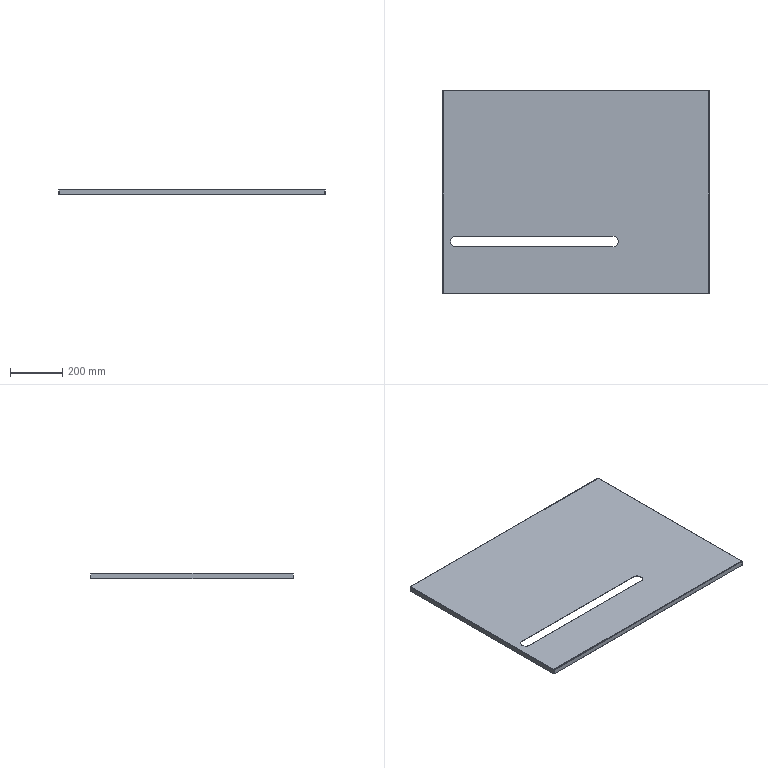Part | STEP file | X77-03009y | 1 solid | 43 faces | box 1018 x 778 x 20 mm | volume 1245859 mm3 | plane 24 | cylinder 11 | spline 8 | commonest cylinder face diameters 1.473 x4 4.473 x4 40 x3